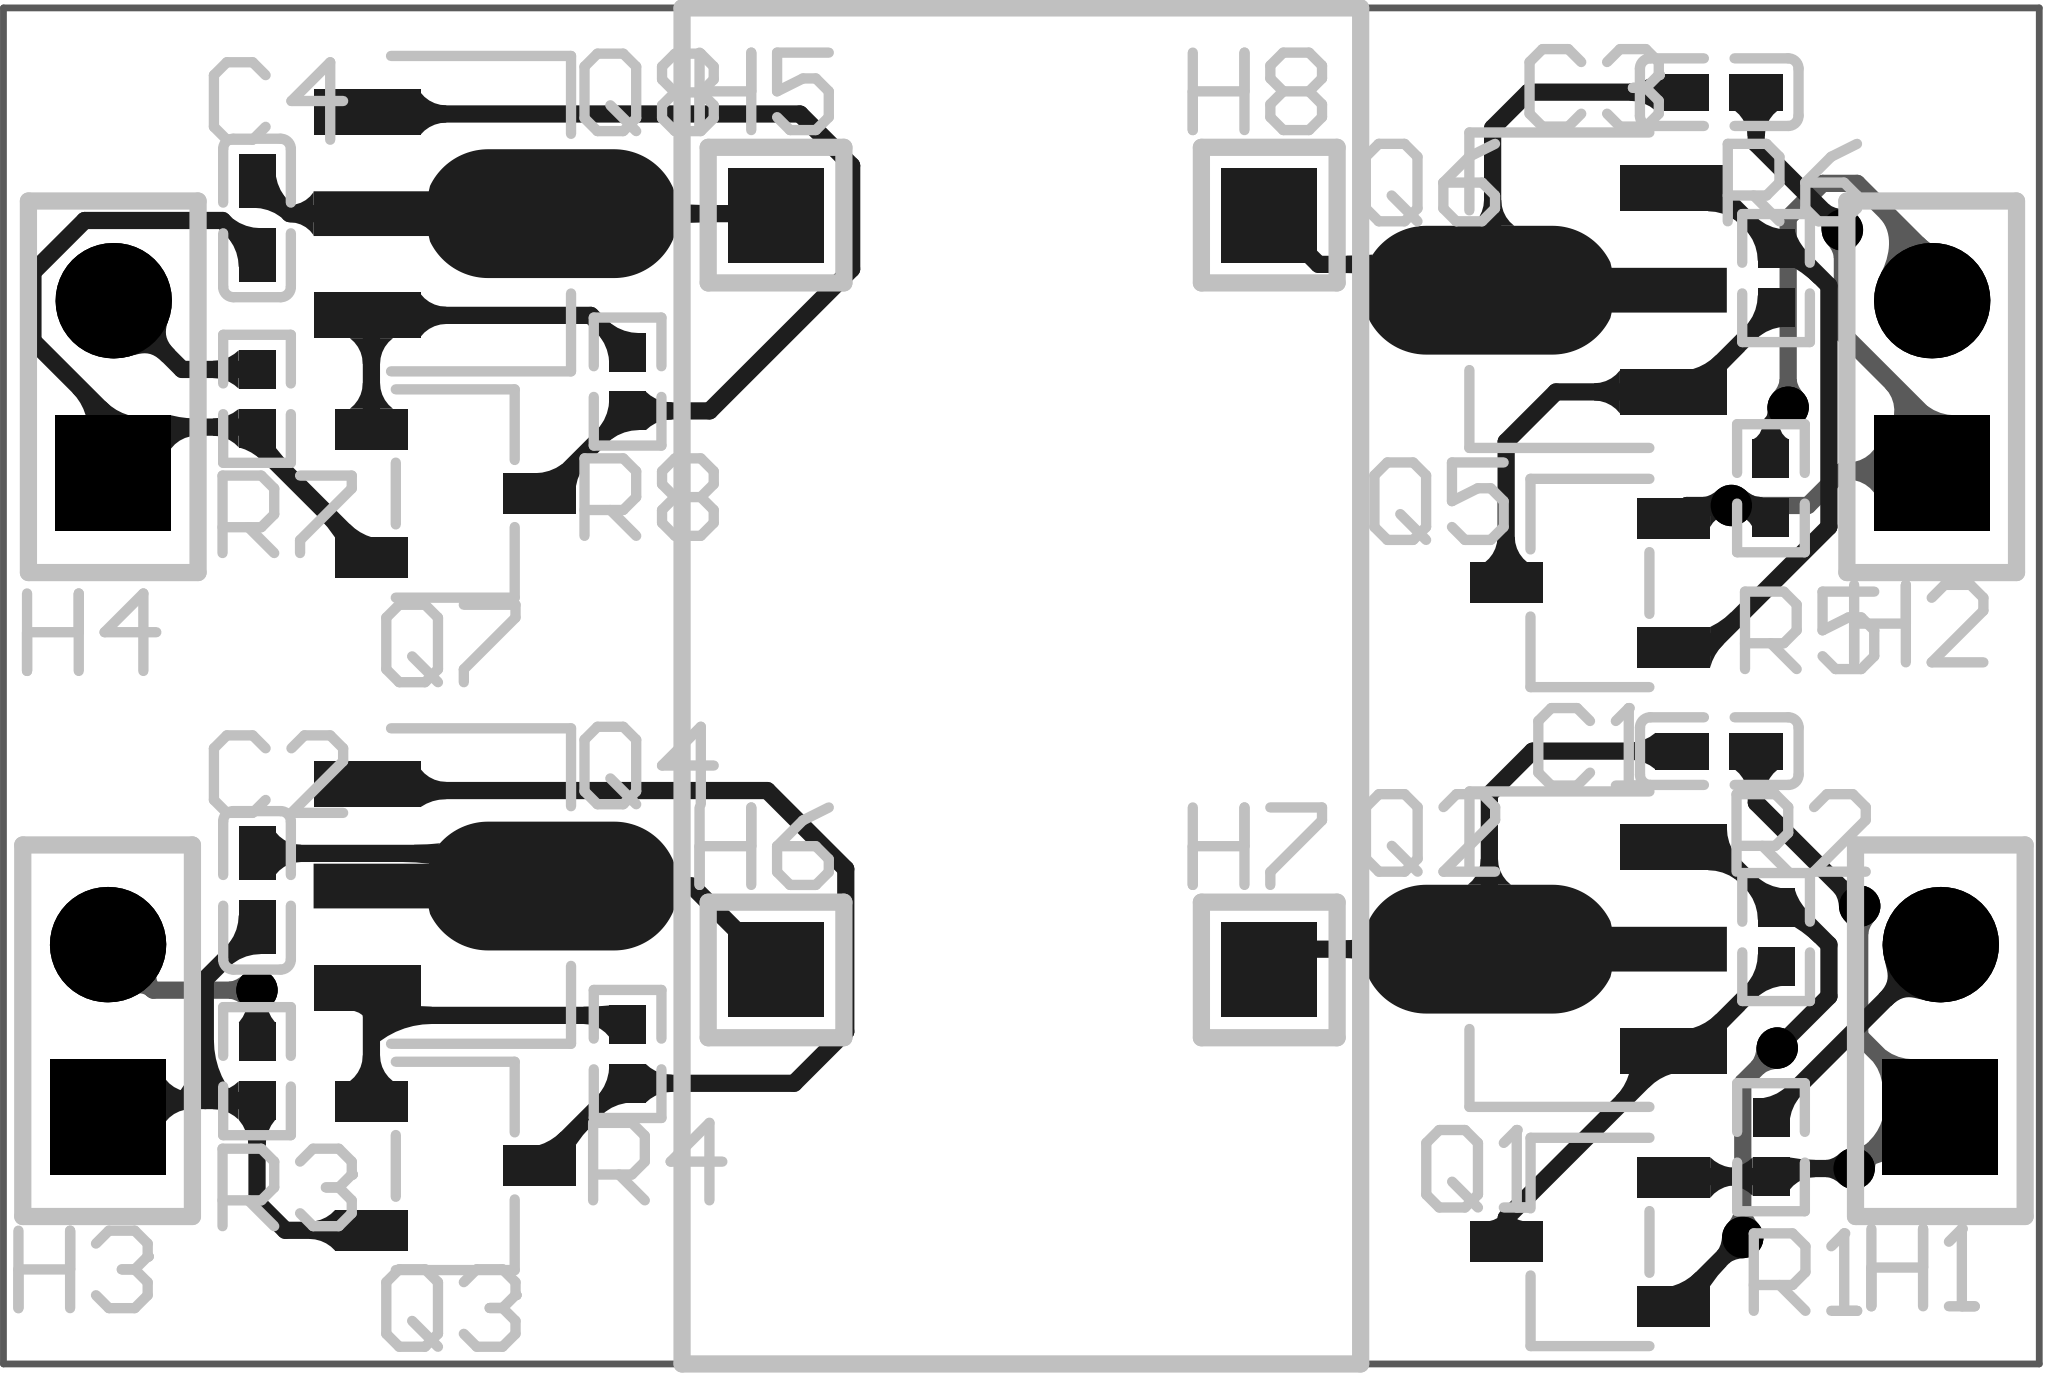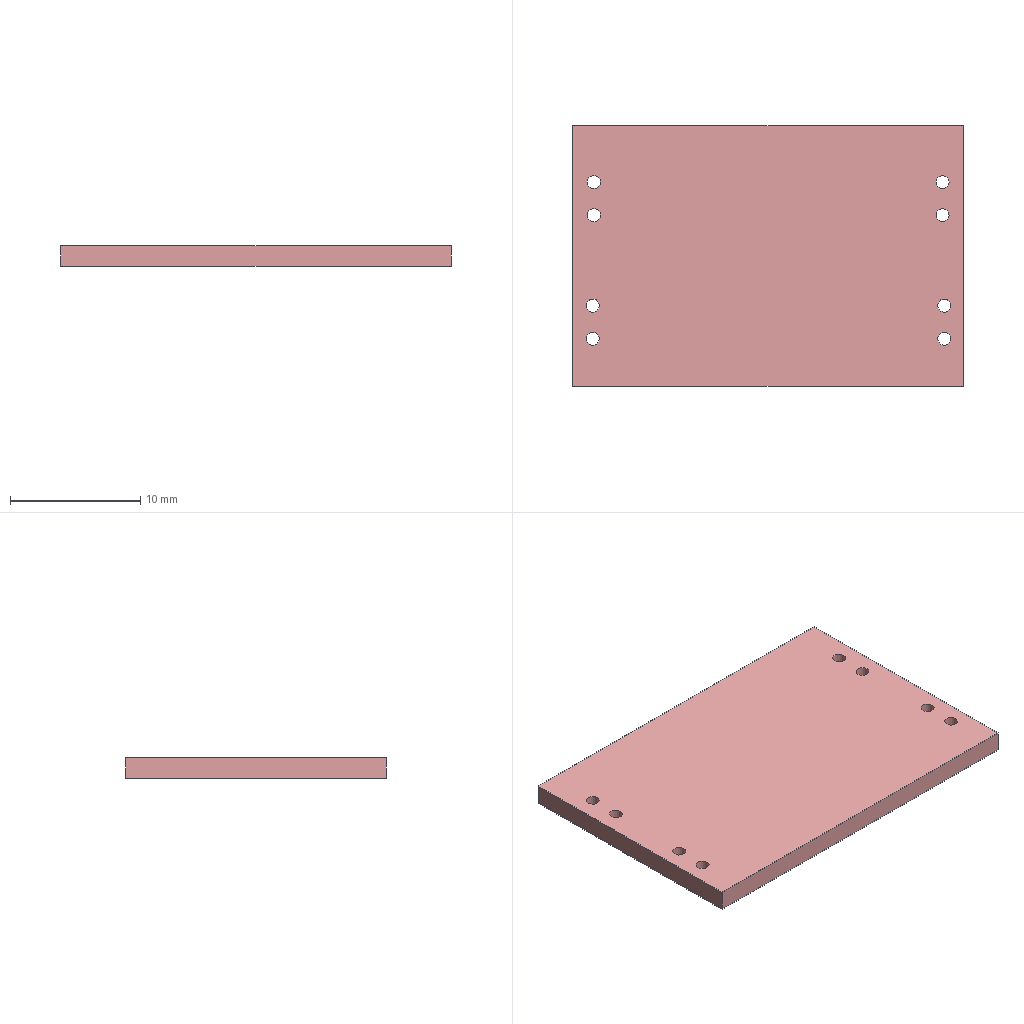Circuit board layout | Altium Designer | box 30 x 20 x 1.6 mm
Layer stack:
# Altium Designer layer stack of  (unit mm; dielectric type: 0 none, 1 core, 2 prepreg, 3 surface material)
index,name,kind,layer,copper_thickness_mm,dielectric_type,dielectric_thickness_mm,dielectric_material,dielectric_constant
0,Top Paste Mask Layer,other,,,,,,
1,Top Silkscreen Layer,other,,,,,,
2,Top Solder Mask Layer,dielectric,,,3,0.01,,3.3
3,Top Layer,copper,Top Layer,0.035,,,,
4,Dielectric1,dielectric,,,3,1.51,FR4,4.5
5,Bottom Layer,copper,Bottom Layer,0.035,,,,
6,Bottom Solder Mask Layer,dielectric,,,3,0.01,,3.3
7,Bottom Silkscreen Layer,other,,,,,,
8,Bottom Paste Mask Layer,other,,,,,,
# drill layer pairs: low layer,high layer
drill_pair,Top Layer,Bottom Layer
Part placement:
Designator,Comment,Layer,Footprint,Center-X(mm),Center-Y(mm),Rotation
C1,1nF,TopLayer,C0402,101.485,85.239,0
C2,1nF,TopLayer,C0402,79.936,83.185,270
C3,1nF,TopLayer,C0402,101.484,94.957,0
C4,1nF,TopLayer,C0402,79.936,93.102,270
Q1,BC856B,TopLayer,SOT-23-3_L2.9-W1.6-P1.90-LS2.8-BR,99.58,78,0
Q2,2N2222AU,TopLayer,SOT-89-3_L4.5-W2.4-P1.50-LS4.0-BR,99.648,82.318,0
Q3,BC856B,TopLayer,SOT-23-3_L2.9-W1.6-P1.90-LS2.8-BR,82.858,79.121,180
Q4,2N2222AU,TopLayer,SOT-89-3_L4.5-W2.4-P1.50-LS4.0-BR,82.719,83.249,180
Q5,BC856B,TopLayer,SOT-23-3_L2.9-W1.6-P1.90-LS2.8-BR,99.579,87.719,0
Q6,2N2222AU,TopLayer,SOT-89-3_L4.5-W2.4-P1.50-LS4.0-BR,99.647,92.037,0
Q7,BC856B,TopLayer,SOT-23-3_L2.9-W1.6-P1.90-LS2.8-BR,82.858,89.038,180
Q8,2N2222AU,TopLayer,SOT-89-3_L4.5-W2.4-P1.50-LS4.0-BR,82.719,93.165,180
R1,3.9K,TopLayer,R0402,102.247,79.397,270
R2,200k,TopLayer,R0402,102.322,82.496,90
R3,3.9K,TopLayer,R0402,79.936,80.518,270
R4,200k,TopLayer,R0402,85.397,80.772,90
R5,3.9K,TopLayer,R0402,102.246,89.115,270
R6,200k,TopLayer,R0402,102.321,92.215,90
R7,3.9K,TopLayer,R0402,79.936,90.435,270
R8,200k,TopLayer,R0402,85.397,90.689,90
H1,,TopLayer,HDR-TH_2P-P2.54-V-F,104.742,81.115,90
H2,,TopLayer,HDR-TH_2P-P2.54-V-F,104.615,90.612,90
H3,,TopLayer,HDR-TH_2P-P2.54-V-F,77.735,81.115,90
H4,,TopLayer,HDR-TH_2P-P2.54-V-F,77.818,90.612,90
H5,,TopLayer,HDR-TH_1P-V-M_XKB_X4611WV-01I-C28D40,87.585,93.144,0
H6,,TopLayer,HDR-TH_1P-V-M_XKB_X4611WV-01I-C28D40,87.585,82.011,0
H7,,TopLayer,HDR-TH_1P-V-M_XKB_X4611WV-01I-C28D40,94.853,82.011,0
H8,,TopLayer,HDR-TH_1P-V-M_XKB_X4611WV-01I-C28D40,94.853,93.144,0
Pad and via stacks:
# Altium Designer via and pad stacks of  (unit mm). Each distinct definition once, with the count of objects using it.
# via: kind,start_layer,end_layer,hole_mm,diameter_mm,mode(0 simple;1 top-mid-bottom;2 full stack),diameter_per_layer,count,example_net
# pad: kind,layer,hole_mm,hole_type(0 round;1 square;2 slot),plating,top_size,top_shape(1 round;2 rect;3 octagon;9 rounded rect),mid_size,bottom_size,mode,footprint,size_per_layer,count,example
pad,Top Layer,0,0,plated,0.7901x0.54,2,0.7901x0.54,0.7901x0.54,0,C0402,,8,C1.2
pad,Top Layer,0,0,plated,1.07x0.6,2,1.07x0.6,1.07x0.6,0,SOT-23-3_L2.9-W1.6-P1.90-LS2.8-BR,,12,Q1.1
pad,Top Layer,0,0,plated,0.95x0.95,1,0.95x0.95,0.95x0.95,0,SOT-89-3_L4.5-W2.4-P1.50-LS4.0-BR,,4,Q2.2
pad,Top Layer,0,0,plated,1.575x0.672,2,1.575x0.672,1.575x0.672,0,SOT-89-3_L4.5-W2.4-P1.50-LS4.0-BR,,8,Q2.3
pad,Top Layer,0,0,plated,0.5657x0.54,2,0.5657x0.54,0.5657x0.54,0,R0402,,16,R1.2
pad,Top Layer,0,0,plated,1.4x1.4,2,1.4x1.4,1.4x1.4,0,HDR-TH_1P-V-M_XKB_X4611WV-01I-C28D40,,4,H5.1
pad,Multi-Layer,1,0,plated,1.7x1.7,2,1.7x1.7,1.7x1.7,0,HDR-TH_2P-P2.54-V-F,,4,H1.1
pad,Multi-Layer,1,0,plated,1.7x1.7,1,1.7x1.7,1.7x1.7,0,HDR-TH_2P-P2.54-V-F,,4,H1.2
via,Top Layer,Bottom Layer,0.3048,0.61,0,,8,$1N634